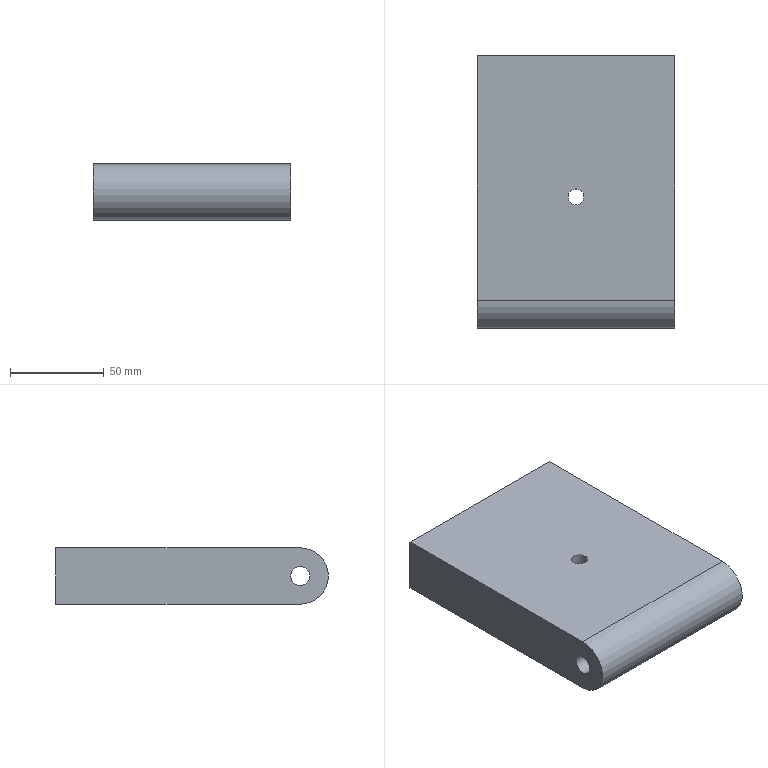Part | STEP file | gslz 2016.10.28-13_id1862_x_t | 1 solid | 8 faces | box 105 x 145.1 x 30 mm | volume 436893 mm3 | plane 5 | cylinder 3 | commonest cylinder face diameters 8.5 x1 10.05 x1 30 x1
STEP:
#1=CARTESIAN_POINT('',(0.,0.,0.));
#2=DIRECTION('',(0.,0.,1.));
#3=DIRECTION('',(1.,0.,0.));
#4=AXIS2_PLACEMENT_3D('',#1,#2,#3);
#5=CARTESIAN_POINT('',(1182.5,600.1,-49.));
#6=VERTEX_POINT('',#5);
#7=CARTESIAN_POINT('',(1182.5,730.2,-49.));
#8=VERTEX_POINT('',#7);
#9=CARTESIAN_POINT('',(1182.5,600.95,-49.));
#10=DIRECTION('',(0.,1.,0.));
#11=VECTOR('',#10,1.);
#12=LINE('',#9,#11);
#13=CARTESIAN_POINT('',(1322.5,601.2,-49.));
#14=DIRECTION('',(0.,0.,-1.));
#15=DIRECTION('',(0.,1.,0.));
#16=AXIS2_PLACEMENT_3D('',#13,#14,#15);
#17=PLANE('',#16);
#18=CARTESIAN_POINT('',(-0.25,-140.));
#19=DIRECTION('',(1.,0.));
#20=VECTOR('',#19,1.);
#21=LINE('',#18,#20);
#22=(GEOMETRIC_REPRESENTATION_CONTEXT(2)PARAMETRIC_REPRESENTATION_CONTEXT()REPRESENTATION_CONTEXT('',''));
#23=DEFINITIONAL_REPRESENTATION('',(#21),#22);
#24=PCURVE('',#17,#23);
#25=CARTESIAN_POINT('',(1182.5,600.95,-69.));
#26=DIRECTION('',(1.,0.,0.));
#27=DIRECTION('',(0.,0.,1.));
#28=AXIS2_PLACEMENT_3D('',#25,#26,#27);
#29=PLANE('',#28);
#30=CARTESIAN_POINT('',(20.,0.));
#31=DIRECTION('',(0.,-1.));
#32=VECTOR('',#31,1.);
#33=LINE('',#30,#32);
#34=(GEOMETRIC_REPRESENTATION_CONTEXT(2)PARAMETRIC_REPRESENTATION_CONTEXT()REPRESENTATION_CONTEXT('',''));
#35=DEFINITIONAL_REPRESENTATION('',(#33),#34);
#36=PCURVE('',#29,#35);
#37=SURFACE_CURVE('',#12,(#24,#36),.PCURVE_S1.);
#38=EDGE_CURVE('',#6,#8,#37,.T.);
#39=ORIENTED_EDGE('',*,*,#38,.F.);
#40=CARTESIAN_POINT('',(1287.5,600.1,-49.));
#41=VERTEX_POINT('',#40);
#42=CARTESIAN_POINT('',(1235.,600.1,-49.));
#43=DIRECTION('',(1.,0.,0.));
#44=VECTOR('',#43,1.);
#45=LINE('',#42,#44);
#46=CARTESIAN_POINT('',(-1.1,-87.5));
#47=DIRECTION('',(0.,1.));
#48=VECTOR('',#47,1.);
#49=LINE('',#46,#48);
#50=(GEOMETRIC_REPRESENTATION_CONTEXT(2)PARAMETRIC_REPRESENTATION_CONTEXT()REPRESENTATION_CONTEXT('',''));
#51=DEFINITIONAL_REPRESENTATION('',(#49),#50);
#52=PCURVE('',#17,#51);
#53=CARTESIAN_POINT('',(1322.5,600.1,-64.));
#54=DIRECTION('',(-1.,0.,0.));
#55=DIRECTION('',(0.,0.,1.));
#56=AXIS2_PLACEMENT_3D('',#53,#54,#55);
#57=CYLINDRICAL_SURFACE('',#56,15.);
#58=CARTESIAN_POINT('',(6.283,87.5));
#59=DIRECTION('',(0.,-1.));
#60=VECTOR('',#59,1.);
#61=LINE('',#58,#60);
#62=(GEOMETRIC_REPRESENTATION_CONTEXT(2)PARAMETRIC_REPRESENTATION_CONTEXT()REPRESENTATION_CONTEXT('',''));
#63=DEFINITIONAL_REPRESENTATION('',(#61),#62);
#64=PCURVE('',#57,#63);
#65=SURFACE_CURVE('',#45,(#52,#64),.PCURVE_S1.);
#66=EDGE_CURVE('',#6,#41,#65,.T.);
#67=ORIENTED_EDGE('',*,*,#66,.T.);
#68=CARTESIAN_POINT('',(1287.5,730.2,-49.));
#69=VERTEX_POINT('',#68);
#70=CARTESIAN_POINT('',(1287.5,600.95,-49.));
#71=DIRECTION('',(0.,-1.,0.));
#72=VECTOR('',#71,1.);
#73=LINE('',#70,#72);
#74=CARTESIAN_POINT('',(-0.25,-35.));
#75=DIRECTION('',(-1.,0.));
#76=VECTOR('',#75,1.);
#77=LINE('',#74,#76);
#78=(GEOMETRIC_REPRESENTATION_CONTEXT(2)PARAMETRIC_REPRESENTATION_CONTEXT()REPRESENTATION_CONTEXT('',''));
#79=DEFINITIONAL_REPRESENTATION('',(#77),#78);
#80=PCURVE('',#17,#79);
#81=CARTESIAN_POINT('',(1287.5,600.95,-69.));
#82=DIRECTION('',(-1.,0.,0.));
#83=DIRECTION('',(0.,0.,1.));
#84=AXIS2_PLACEMENT_3D('',#81,#82,#83);
#85=PLANE('',#84);
#86=CARTESIAN_POINT('',(20.,0.));
#87=DIRECTION('',(0.,-1.));
#88=VECTOR('',#87,1.);
#89=LINE('',#86,#88);
#90=(GEOMETRIC_REPRESENTATION_CONTEXT(2)PARAMETRIC_REPRESENTATION_CONTEXT()REPRESENTATION_CONTEXT('',''));
#91=DEFINITIONAL_REPRESENTATION('',(#89),#90);
#92=PCURVE('',#85,#91);
#93=SURFACE_CURVE('',#73,(#80,#92),.PCURVE_S1.);
#94=EDGE_CURVE('',#69,#41,#93,.T.);
#95=ORIENTED_EDGE('',*,*,#94,.F.);
#96=CARTESIAN_POINT('',(1322.5,730.2,-49.));
#97=DIRECTION('',(-1.,0.,0.));
#98=VECTOR('',#97,1.);
#99=LINE('',#96,#98);
#100=CARTESIAN_POINT('',(129.,0.));
#101=DIRECTION('',(0.,-1.));
#102=VECTOR('',#101,1.);
#103=LINE('',#100,#102);
#104=(GEOMETRIC_REPRESENTATION_CONTEXT(2)PARAMETRIC_REPRESENTATION_CONTEXT()REPRESENTATION_CONTEXT('',''));
#105=DEFINITIONAL_REPRESENTATION('',(#103),#104);
#106=PCURVE('',#17,#105);
#107=CARTESIAN_POINT('',(1322.5,730.2,-34.));
#108=DIRECTION('',(0.,-1.,0.));
#109=DIRECTION('',(-1.,0.,0.));
#110=AXIS2_PLACEMENT_3D('',#107,#108,#109);
#111=PLANE('',#110);
#112=CARTESIAN_POINT('',(0.,15.));
#113=DIRECTION('',(1.,0.));
#114=VECTOR('',#113,1.);
#115=LINE('',#112,#114);
#116=(GEOMETRIC_REPRESENTATION_CONTEXT(2)PARAMETRIC_REPRESENTATION_CONTEXT()REPRESENTATION_CONTEXT('',''));
#117=DEFINITIONAL_REPRESENTATION('',(#115),#116);
#118=PCURVE('',#111,#117);
#119=SURFACE_CURVE('',#99,(#106,#118),.PCURVE_S1.);
#120=EDGE_CURVE('',#69,#8,#119,.T.);
#121=ORIENTED_EDGE('',*,*,#120,.T.);
#122=EDGE_LOOP('',(#39,#67,#95,#121));
#123=FACE_BOUND('',#122,.T.);
#124=CARTESIAN_POINT('',(1230.75,655.1,-49.));
#125=VERTEX_POINT('',#124);
#126=CARTESIAN_POINT('',(1235.,655.1,-49.));
#127=DIRECTION('',(0.,0.,1.));
#128=DIRECTION('',(-1.,0.,0.));
#129=AXIS2_PLACEMENT_3D('',#126,#127,#128);
#130=CIRCLE('',#129,4.25);
#131=CARTESIAN_POINT('',(53.9,-91.75));
#132=CARTESIAN_POINT('',(46.539,-91.75));
#133=CARTESIAN_POINT('',(50.219,-85.375));
#134=CARTESIAN_POINT('',(53.9,-79.));
#135=CARTESIAN_POINT('',(57.581,-85.375));
#136=CARTESIAN_POINT('',(61.261,-91.75));
#137=CARTESIAN_POINT('',(53.9,-91.75));
#138=(BOUNDED_CURVE()B_SPLINE_CURVE(2,(#131,#132,#133,#134,#135,#136,#137),.UNSPECIFIED.,.T.,.F.)B_SPLINE_CURVE_WITH_KNOTS((1,2,2,2,2,1),(-2.094,0.,2.094,4.189,6.283,8.378),.UNSPECIFIED.)CURVE()GEOMETRIC_REPRESENTATION_ITEM()RATIONAL_B_SPLINE_CURVE((1.,0.5,1.,0.5,1.,0.5,1.))REPRESENTATION_ITEM(''));
#139=(GEOMETRIC_REPRESENTATION_CONTEXT(2)PARAMETRIC_REPRESENTATION_CONTEXT()REPRESENTATION_CONTEXT('',''));
#140=DEFINITIONAL_REPRESENTATION('',(#138),#139);
#141=PCURVE('',#17,#140);
#142=CARTESIAN_POINT('',(1235.,655.1,356.));
#143=DIRECTION('',(0.,0.,-1.));
#144=DIRECTION('',(-1.,0.,0.));
#145=AXIS2_PLACEMENT_3D('',#142,#143,#144);
#146=CYLINDRICAL_SURFACE('',#145,4.25);
#147=CARTESIAN_POINT('',(6.283,405.));
#148=DIRECTION('',(-1.,0.));
#149=VECTOR('',#148,1.);
#150=LINE('',#147,#149);
#151=(GEOMETRIC_REPRESENTATION_CONTEXT(2)PARAMETRIC_REPRESENTATION_CONTEXT()REPRESENTATION_CONTEXT('',''));
#152=DEFINITIONAL_REPRESENTATION('',(#150),#151);
#153=PCURVE('',#146,#152);
#154=SURFACE_CURVE('',#130,(#141,#153),.PCURVE_S1.);
#155=EDGE_CURVE('',#125,#125,#154,.T.);
#156=ORIENTED_EDGE('',*,*,#155,.F.);
#157=EDGE_LOOP('',(#156));
#158=FACE_BOUND('',#157,.T.);
#159=ADVANCED_FACE('',(#123,#158),#17,.F.);
#160=CARTESIAN_POINT('',(1287.5,600.1,-79.));
#161=VERTEX_POINT('',#160);
#162=CARTESIAN_POINT('',(1287.5,730.2,-79.));
#163=VERTEX_POINT('',#162);
#164=CARTESIAN_POINT('',(1287.5,600.95,-79.));
#165=DIRECTION('',(0.,1.,0.));
#166=VECTOR('',#165,1.);
#167=LINE('',#164,#166);
#168=CARTESIAN_POINT('',(1322.5,581.2,-79.));
#169=DIRECTION('',(0.,0.,1.));
#170=DIRECTION('',(0.,-1.,0.));
#171=AXIS2_PLACEMENT_3D('',#168,#169,#170);
#172=PLANE('',#171);
#173=CARTESIAN_POINT('',(-19.75,-35.));
#174=DIRECTION('',(-1.,0.));
#175=VECTOR('',#174,1.);
#176=LINE('',#173,#175);
#177=(GEOMETRIC_REPRESENTATION_CONTEXT(2)PARAMETRIC_REPRESENTATION_CONTEXT()REPRESENTATION_CONTEXT('',''));
#178=DEFINITIONAL_REPRESENTATION('',(#176),#177);
#179=PCURVE('',#172,#178);
#180=CARTESIAN_POINT('',(-10.,0.));
#181=DIRECTION('',(0.,1.));
#182=VECTOR('',#181,1.);
#183=LINE('',#180,#182);
#184=(GEOMETRIC_REPRESENTATION_CONTEXT(2)PARAMETRIC_REPRESENTATION_CONTEXT()REPRESENTATION_CONTEXT('',''));
#185=DEFINITIONAL_REPRESENTATION('',(#183),#184);
#186=PCURVE('',#85,#185);
#187=SURFACE_CURVE('',#167,(#179,#186),.PCURVE_S1.);
#188=EDGE_CURVE('',#161,#163,#187,.T.);
#189=ORIENTED_EDGE('',*,*,#188,.F.);
#190=CARTESIAN_POINT('',(1182.5,600.1,-79.));
#191=VERTEX_POINT('',#190);
#192=CARTESIAN_POINT('',(1235.,600.1,-79.));
#193=DIRECTION('',(-1.,0.,0.));
#194=VECTOR('',#193,1.);
#195=LINE('',#192,#194);
#196=CARTESIAN_POINT('',(-18.9,-87.5));
#197=DIRECTION('',(0.,-1.));
#198=VECTOR('',#197,1.);
#199=LINE('',#196,#198);
#200=(GEOMETRIC_REPRESENTATION_CONTEXT(2)PARAMETRIC_REPRESENTATION_CONTEXT()REPRESENTATION_CONTEXT('',''));
#201=DEFINITIONAL_REPRESENTATION('',(#199),#200);
#202=PCURVE('',#172,#201);
#203=CARTESIAN_POINT('',(3.142,87.5));
#204=DIRECTION('',(0.,1.));
#205=VECTOR('',#204,1.);
#206=LINE('',#203,#205);
#207=(GEOMETRIC_REPRESENTATION_CONTEXT(2)PARAMETRIC_REPRESENTATION_CONTEXT()REPRESENTATION_CONTEXT('',''));
#208=DEFINITIONAL_REPRESENTATION('',(#206),#207);
#209=PCURVE('',#57,#208);
#210=SURFACE_CURVE('',#195,(#202,#209),.PCURVE_S1.);
#211=EDGE_CURVE('',#161,#191,#210,.T.);
#212=ORIENTED_EDGE('',*,*,#211,.T.);
#213=CARTESIAN_POINT('',(1182.5,730.2,-79.));
#214=VERTEX_POINT('',#213);
#215=CARTESIAN_POINT('',(1182.5,581.2,-79.));
#216=DIRECTION('',(0.,1.,0.));
#217=VECTOR('',#216,1.);
#218=LINE('',#215,#217);
#219=CARTESIAN_POINT('',(0.,-140.));
#220=DIRECTION('',(-1.,0.));
#221=VECTOR('',#220,1.);
#222=LINE('',#219,#221);
#223=(GEOMETRIC_REPRESENTATION_CONTEXT(2)PARAMETRIC_REPRESENTATION_CONTEXT()REPRESENTATION_CONTEXT('',''));
#224=DEFINITIONAL_REPRESENTATION('',(#222),#223);
#225=PCURVE('',#172,#224);
#226=CARTESIAN_POINT('',(-10.,19.75));
#227=DIRECTION('',(0.,-1.));
#228=VECTOR('',#227,1.);
#229=LINE('',#226,#228);
#230=(GEOMETRIC_REPRESENTATION_CONTEXT(2)PARAMETRIC_REPRESENTATION_CONTEXT()REPRESENTATION_CONTEXT('',''));
#231=DEFINITIONAL_REPRESENTATION('',(#229),#230);
#232=PCURVE('',#29,#231);
#233=SURFACE_CURVE('',#218,(#225,#232),.PCURVE_S1.);
#234=EDGE_CURVE('',#191,#214,#233,.T.);
#235=ORIENTED_EDGE('',*,*,#234,.T.);
#236=CARTESIAN_POINT('',(1322.5,730.2,-79.));
#237=DIRECTION('',(-1.,0.,0.));
#238=VECTOR('',#237,1.);
#239=LINE('',#236,#238);
#240=CARTESIAN_POINT('',(-149.,0.));
#241=DIRECTION('',(0.,-1.));
#242=VECTOR('',#241,1.);
#243=LINE('',#240,#242);
#244=(GEOMETRIC_REPRESENTATION_CONTEXT(2)PARAMETRIC_REPRESENTATION_CONTEXT()REPRESENTATION_CONTEXT('',''));
#245=DEFINITIONAL_REPRESENTATION('',(#243),#244);
#246=PCURVE('',#172,#245);
#247=CARTESIAN_POINT('',(0.,45.));
#248=DIRECTION('',(1.,0.));
#249=VECTOR('',#248,1.);
#250=LINE('',#247,#249);
#251=(GEOMETRIC_REPRESENTATION_CONTEXT(2)PARAMETRIC_REPRESENTATION_CONTEXT()REPRESENTATION_CONTEXT('',''));
#252=DEFINITIONAL_REPRESENTATION('',(#250),#251);
#253=PCURVE('',#111,#252);
#254=SURFACE_CURVE('',#239,(#246,#253),.PCURVE_S1.);
#255=EDGE_CURVE('',#163,#214,#254,.T.);
#256=ORIENTED_EDGE('',*,*,#255,.F.);
#257=EDGE_LOOP('',(#189,#212,#235,#256));
#258=FACE_BOUND('',#257,.T.);
#259=CARTESIAN_POINT('',(1239.25,655.1,-79.));
#260=VERTEX_POINT('',#259);
#261=CARTESIAN_POINT('',(1230.75,655.1,-79.));
#262=VERTEX_POINT('',#261);
#263=CARTESIAN_POINT('',(1235.,655.1,-79.));
#264=DIRECTION('',(0.,0.,-1.));
#265=DIRECTION('',(1.,0.,0.));
#266=AXIS2_PLACEMENT_3D('',#263,#264,#265);
#267=CIRCLE('',#266,4.25);
#268=CARTESIAN_POINT('',(-73.9,-83.25));
#269=CARTESIAN_POINT('',(-66.539,-83.25));
#270=CARTESIAN_POINT('',(-70.219,-89.625));
#271=CARTESIAN_POINT('',(-73.9,-96.));
#272=CARTESIAN_POINT('',(-77.581,-89.625));
#273=CARTESIAN_POINT('',(-81.261,-83.25));
#274=CARTESIAN_POINT('',(-73.9,-83.25));
#275=(BOUNDED_CURVE()B_SPLINE_CURVE(2,(#268,#269,#270,#271,#272,#273,#274),.UNSPECIFIED.,.T.,.F.)B_SPLINE_CURVE_WITH_KNOTS((1,2,2,2,2,1),(-2.094,0.,2.094,4.189,6.283,8.378),.UNSPECIFIED.)CURVE()GEOMETRIC_REPRESENTATION_ITEM()RATIONAL_B_SPLINE_CURVE((1.,0.5,1.,0.5,1.,0.5,1.))REPRESENTATION_ITEM(''));
#276=(GEOMETRIC_REPRESENTATION_CONTEXT(2)PARAMETRIC_REPRESENTATION_CONTEXT()REPRESENTATION_CONTEXT('',''));
#277=DEFINITIONAL_REPRESENTATION('',(#275),#276);
#278=PCURVE('',#172,#277);
#279=CARTESIAN_POINT('',(3.142,435.));
#280=DIRECTION('',(1.,0.));
#281=VECTOR('',#280,1.);
#282=LINE('',#279,#281);
#283=(GEOMETRIC_REPRESENTATION_CONTEXT(2)PARAMETRIC_REPRESENTATION_CONTEXT()REPRESENTATION_CONTEXT('',''));
#284=DEFINITIONAL_REPRESENTATION('',(#282),#283);
#285=PCURVE('',#146,#284);
#286=SURFACE_CURVE('',#267,(#278,#285),.PCURVE_S1.);
#287=EDGE_CURVE('',#260,#262,#286,.T.);
#288=ORIENTED_EDGE('',*,*,#287,.F.);
#289=CARTESIAN_POINT('',(1235.,655.1,-79.));
#290=DIRECTION('',(0.,0.,-1.));
#291=DIRECTION('',(1.,0.,0.));
#292=AXIS2_PLACEMENT_3D('',#289,#290,#291);
#293=CIRCLE('',#292,4.25);
#294=CARTESIAN_POINT('',(-73.9,-83.25));
#295=CARTESIAN_POINT('',(-66.539,-83.25));
#296=CARTESIAN_POINT('',(-70.219,-89.625));
#297=CARTESIAN_POINT('',(-73.9,-96.));
#298=CARTESIAN_POINT('',(-77.581,-89.625));
#299=CARTESIAN_POINT('',(-81.261,-83.25));
#300=CARTESIAN_POINT('',(-73.9,-83.25));
#301=(BOUNDED_CURVE()B_SPLINE_CURVE(2,(#294,#295,#296,#297,#298,#299,#300),.UNSPECIFIED.,.T.,.F.)B_SPLINE_CURVE_WITH_KNOTS((1,2,2,2,2,1),(-2.094,0.,2.094,4.189,6.283,8.378),.UNSPECIFIED.)CURVE()GEOMETRIC_REPRESENTATION_ITEM()RATIONAL_B_SPLINE_CURVE((1.,0.5,1.,0.5,1.,0.5,1.))REPRESENTATION_ITEM(''));
#302=(GEOMETRIC_REPRESENTATION_CONTEXT(2)PARAMETRIC_REPRESENTATION_CONTEXT()REPRESENTATION_CONTEXT('',''));
#303=DEFINITIONAL_REPRESENTATION('',(#301),#302);
#304=PCURVE('',#172,#303);
#305=CARTESIAN_POINT('',(-3.142,435.));
#306=DIRECTION('',(1.,0.));
#307=VECTOR('',#306,1.);
#308=LINE('',#305,#307);
#309=(GEOMETRIC_REPRESENTATION_CONTEXT(2)PARAMETRIC_REPRESENTATION_CONTEXT()REPRESENTATION_CONTEXT('',''));
#310=DEFINITIONAL_REPRESENTATION('',(#308),#309);
#311=PCURVE('',#146,#310);
#312=SURFACE_CURVE('',#293,(#304,#311),.PCURVE_S1.);
#313=EDGE_CURVE('',#262,#260,#312,.T.);
#314=ORIENTED_EDGE('',*,*,#313,.F.);
#315=EDGE_LOOP('',(#288,#314));
#316=FACE_BOUND('',#315,.T.);
#317=ADVANCED_FACE('',(#258,#316),#172,.F.);
#318=CARTESIAN_POINT('',(1287.5,600.1,-64.));
#319=DIRECTION('',(1.,0.,0.));
#320=DIRECTION('',(0.,0.,1.));
#321=AXIS2_PLACEMENT_3D('',#318,#319,#320);
#322=CIRCLE('',#321,15.);
#323=CARTESIAN_POINT('',(20.,-0.85));
#324=CARTESIAN_POINT('',(20.,-26.831));
#325=CARTESIAN_POINT('',(-2.5,-13.84));
#326=CARTESIAN_POINT('',(-25.,-0.85));
#327=CARTESIAN_POINT('',(-2.5,12.14));
#328=CARTESIAN_POINT('',(20.,25.131));
#329=CARTESIAN_POINT('',(20.,-0.85));
#330=(BOUNDED_CURVE()B_SPLINE_CURVE(2,(#323,#324,#325,#326,#327,#328,#329),.UNSPECIFIED.,.T.,.F.)B_SPLINE_CURVE_WITH_KNOTS((1,2,2,2,2,1),(-2.094,0.,2.094,4.189,6.283,8.378),.UNSPECIFIED.)CURVE()GEOMETRIC_REPRESENTATION_ITEM()RATIONAL_B_SPLINE_CURVE((1.,0.5,1.,0.5,1.,0.5,1.))REPRESENTATION_ITEM(''));
#331=(GEOMETRIC_REPRESENTATION_CONTEXT(2)PARAMETRIC_REPRESENTATION_CONTEXT()REPRESENTATION_CONTEXT('',''));
#332=DEFINITIONAL_REPRESENTATION('',(#330),#331);
#333=PCURVE('',#85,#332);
#334=CARTESIAN_POINT('',(6.283,35.));
#335=DIRECTION('',(-1.,0.));
#336=VECTOR('',#335,1.);
#337=LINE('',#334,#336);
#338=(GEOMETRIC_REPRESENTATION_CONTEXT(2)PARAMETRIC_REPRESENTATION_CONTEXT()REPRESENTATION_CONTEXT('',''));
#339=DEFINITIONAL_REPRESENTATION('',(#337),#338);
#340=PCURVE('',#57,#339);
#341=SURFACE_CURVE('',#322,(#333,#340),.PCURVE_S1.);
#342=EDGE_CURVE('',#41,#161,#341,.T.);
#343=ORIENTED_EDGE('',*,*,#342,.T.);
#344=ORIENTED_EDGE('',*,*,#188,.T.);
#345=CARTESIAN_POINT('',(1287.5,730.2,-34.));
#346=DIRECTION('',(0.,0.,-1.));
#347=VECTOR('',#346,1.);
#348=LINE('',#345,#347);
#349=CARTESIAN_POINT('',(35.,129.25));
#350=DIRECTION('',(-1.,0.));
#351=VECTOR('',#350,1.);
#352=LINE('',#349,#351);
#353=(GEOMETRIC_REPRESENTATION_CONTEXT(2)PARAMETRIC_REPRESENTATION_CONTEXT()REPRESENTATION_CONTEXT('',''));
#354=DEFINITIONAL_REPRESENTATION('',(#352),#353);
#355=PCURVE('',#85,#354);
#356=CARTESIAN_POINT('',(35.,0.));
#357=DIRECTION('',(0.,1.));
#358=VECTOR('',#357,1.);
#359=LINE('',#356,#358);
#360=(GEOMETRIC_REPRESENTATION_CONTEXT(2)PARAMETRIC_REPRESENTATION_CONTEXT()REPRESENTATION_CONTEXT('',''));
#361=DEFINITIONAL_REPRESENTATION('',(#359),#360);
#362=PCURVE('',#111,#361);
#363=SURFACE_CURVE('',#348,(#355,#362),.PCURVE_S1.);
#364=EDGE_CURVE('',#69,#163,#363,.T.);
#365=ORIENTED_EDGE('',*,*,#364,.F.);
#366=ORIENTED_EDGE('',*,*,#94,.T.);
#367=EDGE_LOOP('',(#343,#344,#365,#366));
#368=FACE_BOUND('',#367,.T.);
#369=CARTESIAN_POINT('',(1287.5,600.1,-58.975));
#370=VERTEX_POINT('',#369);
#371=CARTESIAN_POINT('',(1287.5,600.1,-64.));
#372=DIRECTION('',(1.,0.,0.));
#373=DIRECTION('',(0.,0.,1.));
#374=AXIS2_PLACEMENT_3D('',#371,#372,#373);
#375=CIRCLE('',#374,5.025);
#376=CARTESIAN_POINT('',(10.025,-0.85));
#377=CARTESIAN_POINT('',(10.025,-9.554));
#378=CARTESIAN_POINT('',(2.488,-5.202));
#379=CARTESIAN_POINT('',(-5.05,-0.85));
#380=CARTESIAN_POINT('',(2.488,3.502));
#381=CARTESIAN_POINT('',(10.025,7.854));
#382=CARTESIAN_POINT('',(10.025,-0.85));
#383=(BOUNDED_CURVE()B_SPLINE_CURVE(2,(#376,#377,#378,#379,#380,#381,#382),.UNSPECIFIED.,.T.,.F.)B_SPLINE_CURVE_WITH_KNOTS((1,2,2,2,2,1),(-2.094,0.,2.094,4.189,6.283,8.378),.UNSPECIFIED.)CURVE()GEOMETRIC_REPRESENTATION_ITEM()RATIONAL_B_SPLINE_CURVE((1.,0.5,1.,0.5,1.,0.5,1.))REPRESENTATION_ITEM(''));
#384=(GEOMETRIC_REPRESENTATION_CONTEXT(2)PARAMETRIC_REPRESENTATION_CONTEXT()REPRESENTATION_CONTEXT('',''));
#385=DEFINITIONAL_REPRESENTATION('',(#383),#384);
#386=PCURVE('',#85,#385);
#387=CARTESIAN_POINT('',(1330.,600.1,-64.));
#388=DIRECTION('',(-1.,0.,0.));
#389=DIRECTION('',(0.,0.,1.));
#390=AXIS2_PLACEMENT_3D('',#387,#388,#389);
#391=CYLINDRICAL_SURFACE('',#390,5.025);
#392=CARTESIAN_POINT('',(6.283,42.5));
#393=DIRECTION('',(-1.,0.));
#394=VECTOR('',#393,1.);
#395=LINE('',#392,#394);
#396=(GEOMETRIC_REPRESENTATION_CONTEXT(2)PARAMETRIC_REPRESENTATION_CONTEXT()REPRESENTATION_CONTEXT('',''));
#397=DEFINITIONAL_REPRESENTATION('',(#395),#396);
#398=PCURVE('',#391,#397);
#399=SURFACE_CURVE('',#375,(#386,#398),.PCURVE_S1.);
#400=EDGE_CURVE('',#370,#370,#399,.T.);
#401=ORIENTED_EDGE('',*,*,#400,.F.);
#402=EDGE_LOOP('',(#401));
#403=FACE_BOUND('',#402,.T.);
#404=ADVANCED_FACE('',(#368,#403),#85,.F.);
#405=ORIENTED_EDGE('',*,*,#234,.F.);
#406=CARTESIAN_POINT('',(1182.5,600.1,-64.));
#407=DIRECTION('',(-1.,0.,0.));
#408=DIRECTION('',(0.,0.,-1.));
#409=AXIS2_PLACEMENT_3D('',#406,#407,#408);
#410=CIRCLE('',#409,15.);
#411=CARTESIAN_POINT('',(-10.,0.85));
#412=CARTESIAN_POINT('',(-10.,26.831));
#413=CARTESIAN_POINT('',(12.5,13.84));
#414=CARTESIAN_POINT('',(35.,0.85));
#415=CARTESIAN_POINT('',(12.5,-12.14));
#416=CARTESIAN_POINT('',(-10.,-25.131));
#417=CARTESIAN_POINT('',(-10.,0.85));
#418=(BOUNDED_CURVE()B_SPLINE_CURVE(2,(#411,#412,#413,#414,#415,#416,#417),.UNSPECIFIED.,.T.,.F.)B_SPLINE_CURVE_WITH_KNOTS((1,2,2,2,2,1),(-2.094,0.,2.094,4.189,6.283,8.378),.UNSPECIFIED.)CURVE()GEOMETRIC_REPRESENTATION_ITEM()RATIONAL_B_SPLINE_CURVE((1.,0.5,1.,0.5,1.,0.5,1.))REPRESENTATION_ITEM(''));
#419=(GEOMETRIC_REPRESENTATION_CONTEXT(2)PARAMETRIC_REPRESENTATION_CONTEXT()REPRESENTATION_CONTEXT('',''));
#420=DEFINITIONAL_REPRESENTATION('',(#418),#419);
#421=PCURVE('',#29,#420);
#422=CARTESIAN_POINT('',(3.142,140.));
#423=DIRECTION('',(1.,0.));
#424=VECTOR('',#423,1.);
#425=LINE('',#422,#424);
#426=(GEOMETRIC_REPRESENTATION_CONTEXT(2)PARAMETRIC_REPRESENTATION_CONTEXT()REPRESENTATION_CONTEXT('',''));
#427=DEFINITIONAL_REPRESENTATION('',(#425),#426);
#428=PCURVE('',#57,#427);
#429=SURFACE_CURVE('',#410,(#421,#428),.PCURVE_S1.);
#430=EDGE_CURVE('',#191,#6,#429,.T.);
#431=ORIENTED_EDGE('',*,*,#430,.T.);
#432=ORIENTED_EDGE('',*,*,#38,.T.);
#433=CARTESIAN_POINT('',(1182.5,730.2,-34.));
#434=DIRECTION('',(0.,0.,1.));
#435=VECTOR('',#434,1.);
#436=LINE('',#433,#435);
#437=CARTESIAN_POINT('',(35.,-129.25));
#438=DIRECTION('',(1.,0.));
#439=VECTOR('',#438,1.);
#440=LINE('',#437,#439);
#441=(GEOMETRIC_REPRESENTATION_CONTEXT(2)PARAMETRIC_REPRESENTATION_CONTEXT()REPRESENTATION_CONTEXT('',''));
#442=DEFINITIONAL_REPRESENTATION('',(#440),#441);
#443=PCURVE('',#29,#442);
#444=CARTESIAN_POINT('',(140.,0.));
#445=DIRECTION('',(0.,-1.));
#446=VECTOR('',#445,1.);
#447=LINE('',#444,#446);
#448=(GEOMETRIC_REPRESENTATION_CONTEXT(2)PARAMETRIC_REPRESENTATION_CONTEXT()REPRESENTATION_CONTEXT('',''));
#449=DEFINITIONAL_REPRESENTATION('',(#447),#448);
#450=PCURVE('',#111,#449);
#451=SURFACE_CURVE('',#436,(#443,#450),.PCURVE_S1.);
#452=EDGE_CURVE('',#214,#8,#451,.T.);
#453=ORIENTED_EDGE('',*,*,#452,.F.);
#454=EDGE_LOOP('',(#405,#431,#432,#453));
#455=FACE_BOUND('',#454,.T.);
#456=CARTESIAN_POINT('',(1182.5,600.1,-69.025));
#457=VERTEX_POINT('',#456);
#458=CARTESIAN_POINT('',(1182.5,600.1,-58.975));
#459=VERTEX_POINT('',#458);
#460=CARTESIAN_POINT('',(1182.5,600.1,-64.));
#461=DIRECTION('',(-1.,0.,0.));
#462=DIRECTION('',(0.,0.,-1.));
#463=AXIS2_PLACEMENT_3D('',#460,#461,#462);
#464=CIRCLE('',#463,5.025);
#465=CARTESIAN_POINT('',(-0.025,0.85));
#466=CARTESIAN_POINT('',(-0.025,9.554));
#467=CARTESIAN_POINT('',(7.513,5.202));
#468=CARTESIAN_POINT('',(15.05,0.85));
#469=CARTESIAN_POINT('',(7.513,-3.502));
#470=CARTESIAN_POINT('',(-0.025,-7.854));
#471=CARTESIAN_POINT('',(-0.025,0.85));
#472=(BOUNDED_CURVE()B_SPLINE_CURVE(2,(#465,#466,#467,#468,#469,#470,#471),.UNSPECIFIED.,.T.,.F.)B_SPLINE_CURVE_WITH_KNOTS((1,2,2,2,2,1),(-2.094,0.,2.094,4.189,6.283,8.378),.UNSPECIFIED.)CURVE()GEOMETRIC_REPRESENTATION_ITEM()RATIONAL_B_SPLINE_CURVE((1.,0.5,1.,0.5,1.,0.5,1.))REPRESENTATION_ITEM(''));
#473=(GEOMETRIC_REPRESENTATION_CONTEXT(2)PARAMETRIC_REPRESENTATION_CONTEXT()REPRESENTATION_CONTEXT('',''));
#474=DEFINITIONAL_REPRESENTATION('',(#472),#473);
#475=PCURVE('',#29,#474);
#476=CARTESIAN_POINT('',(3.142,147.5));
#477=DIRECTION('',(1.,0.));
#478=VECTOR('',#477,1.);
#479=LINE('',#476,#478);
#480=(GEOMETRIC_REPRESENTATION_CONTEXT(2)PARAMETRIC_REPRESENTATION_CONTEXT()REPRESENTATION_CONTEXT('',''));
#481=DEFINITIONAL_REPRESENTATION('',(#479),#480);
#482=PCURVE('',#391,#481);
#483=SURFACE_CURVE('',#464,(#475,#482),.PCURVE_S1.);
#484=EDGE_CURVE('',#457,#459,#483,.T.);
#485=ORIENTED_EDGE('',*,*,#484,.F.);
#486=CARTESIAN_POINT('',(1182.5,600.1,-64.));
#487=DIRECTION('',(-1.,0.,0.));
#488=DIRECTION('',(0.,0.,-1.));
#489=AXIS2_PLACEMENT_3D('',#486,#487,#488);
#490=CIRCLE('',#489,5.025);
#491=CARTESIAN_POINT('',(-0.025,0.85));
#492=CARTESIAN_POINT('',(-0.025,9.554));
#493=CARTESIAN_POINT('',(7.513,5.202));
#494=CARTESIAN_POINT('',(15.05,0.85));
#495=CARTESIAN_POINT('',(7.513,-3.502));
#496=CARTESIAN_POINT('',(-0.025,-7.854));
#497=CARTESIAN_POINT('',(-0.025,0.85));
#498=(BOUNDED_CURVE()B_SPLINE_CURVE(2,(#491,#492,#493,#494,#495,#496,#497),.UNSPECIFIED.,.T.,.F.)B_SPLINE_CURVE_WITH_KNOTS((1,2,2,2,2,1),(-2.094,0.,2.094,4.189,6.283,8.378),.UNSPECIFIED.)CURVE()GEOMETRIC_REPRESENTATION_ITEM()RATIONAL_B_SPLINE_CURVE((1.,0.5,1.,0.5,1.,0.5,1.))REPRESENTATION_ITEM(''));
#499=(GEOMETRIC_REPRESENTATION_CONTEXT(2)PARAMETRIC_REPRESENTATION_CONTEXT()REPRESENTATION_CONTEXT('',''));
#500=DEFINITIONAL_REPRESENTATION('',(#498),#499);
#501=PCURVE('',#29,#500);
#502=CARTESIAN_POINT('',(-3.142,147.5));
#503=DIRECTION('',(1.,0.));
#504=VECTOR('',#503,1.);
#505=LINE('',#502,#504);
#506=(GEOMETRIC_REPRESENTATION_CONTEXT(2)PARAMETRIC_REPRESENTATION_CONTEXT()REPRESENTATION_CONTEXT('',''));
#507=DEFINITIONAL_REPRESENTATION('',(#505),#506);
#508=PCURVE('',#391,#507);
#509=SURFACE_CURVE('',#490,(#501,#508),.PCURVE_S1.);
#510=EDGE_CURVE('',#459,#457,#509,.T.);
#511=ORIENTED_EDGE('',*,*,#510,.F.);
#512=EDGE_LOOP('',(#485,#511));
#513=FACE_BOUND('',#512,.T.);
#514=ADVANCED_FACE('',(#455,#513),#29,.F.);
#515=ORIENTED_EDGE('',*,*,#255,.T.);
#516=ORIENTED_EDGE('',*,*,#452,.T.);
#517=ORIENTED_EDGE('',*,*,#120,.F.);
#518=ORIENTED_EDGE('',*,*,#364,.T.);
#519=EDGE_LOOP('',(#515,#516,#517,#518));
#520=FACE_BOUND('',#519,.T.);
#521=ADVANCED_FACE('',(#520),#111,.F.);
#522=ORIENTED_EDGE('',*,*,#430,.F.);
#523=ORIENTED_EDGE('',*,*,#211,.F.);
#524=ORIENTED_EDGE('',*,*,#342,.F.);
#525=ORIENTED_EDGE('',*,*,#66,.F.);
#526=EDGE_LOOP('',(#522,#523,#524,#525));
#527=FACE_BOUND('',#526,.T.);
#528=ADVANCED_FACE('',(#527),#57,.T.);
#529=ORIENTED_EDGE('',*,*,#510,.F.);
#530=CARTESIAN_POINT('',(1287.5,600.1,-58.975));
#531=CARTESIAN_POINT('',(1182.5,600.1,-58.975));
#532=B_SPLINE_CURVE_WITH_KNOTS('',1,(#530,#531),.UNSPECIFIED.,.F.,.F.,(2,2),(42.5,147.5),.PIECEWISE_BEZIER_KNOTS.);
#533=CARTESIAN_POINT('',(0.,0.));
#534=DIRECTION('',(0.,1.));
#535=VECTOR('',#534,1.);
#536=LINE('',#533,#535);
#537=(GEOMETRIC_REPRESENTATION_CONTEXT(2)PARAMETRIC_REPRESENTATION_CONTEXT()REPRESENTATION_CONTEXT('',''));
#538=DEFINITIONAL_REPRESENTATION('',(#536),#537);
#539=PCURVE('',#391,#538);
#540=CARTESIAN_POINT('',(6.283,0.));
#541=DIRECTION('',(0.,1.));
#542=VECTOR('',#541,1.);
#543=LINE('',#540,#542);
#544=(GEOMETRIC_REPRESENTATION_CONTEXT(2)PARAMETRIC_REPRESENTATION_CONTEXT()REPRESENTATION_CONTEXT('',''));
#545=DEFINITIONAL_REPRESENTATION('',(#543),#544);
#546=PCURVE('',#391,#545);
#547=SEAM_CURVE('',#532,(#539,#546),.PCURVE_S1.);
#548=EDGE_CURVE('',#370,#459,#547,.T.);
#549=ORIENTED_EDGE('',*,*,#548,.F.);
#550=ORIENTED_EDGE('',*,*,#400,.F.);
#551=ORIENTED_EDGE('',*,*,#548,.T.);
#552=ORIENTED_EDGE('',*,*,#484,.F.);
#553=EDGE_LOOP('',(#529,#549,#550,#551,#552));
#554=FACE_BOUND('',#553,.F.);
#555=ADVANCED_FACE('',(#554),#391,.F.);
#556=ORIENTED_EDGE('',*,*,#313,.F.);
#557=CARTESIAN_POINT('',(1230.75,655.1,-49.));
#558=CARTESIAN_POINT('',(1230.75,655.1,-79.));
#559=B_SPLINE_CURVE_WITH_KNOTS('',1,(#557,#558),.UNSPECIFIED.,.F.,.F.,(2,2),(405.,435.),.PIECEWISE_BEZIER_KNOTS.);
#560=CARTESIAN_POINT('',(0.,0.));
#561=DIRECTION('',(0.,1.));
#562=VECTOR('',#561,1.);
#563=LINE('',#560,#562);
#564=(GEOMETRIC_REPRESENTATION_CONTEXT(2)PARAMETRIC_REPRESENTATION_CONTEXT()REPRESENTATION_CONTEXT('',''));
#565=DEFINITIONAL_REPRESENTATION('',(#563),#564);
#566=PCURVE('',#146,#565);
#567=CARTESIAN_POINT('',(6.283,0.));
#568=DIRECTION('',(0.,1.));
#569=VECTOR('',#568,1.);
#570=LINE('',#567,#569);
#571=(GEOMETRIC_REPRESENTATION_CONTEXT(2)PARAMETRIC_REPRESENTATION_CONTEXT()REPRESENTATION_CONTEXT('',''));
#572=DEFINITIONAL_REPRESENTATION('',(#570),#571);
#573=PCURVE('',#146,#572);
#574=SEAM_CURVE('',#559,(#566,#573),.PCURVE_S1.);
#575=EDGE_CURVE('',#125,#262,#574,.T.);
#576=ORIENTED_EDGE('',*,*,#575,.F.);
#577=ORIENTED_EDGE('',*,*,#155,.F.);
#578=ORIENTED_EDGE('',*,*,#575,.T.);
#579=ORIENTED_EDGE('',*,*,#287,.F.);
#580=EDGE_LOOP('',(#556,#576,#577,#578,#579));
#581=FACE_BOUND('',#580,.F.);
#582=ADVANCED_FACE('',(#581),#146,.F.);
#583=CLOSED_SHELL('',(#159,#317,#404,#514,#521,#528,#555,#582));
#584=MANIFOLD_SOLID_BREP('',#583);
#585=(LENGTH_UNIT()NAMED_UNIT(*)SI_UNIT(.MILLI.,.METRE.));
#586=UNCERTAINTY_MEASURE_WITH_UNIT(LENGTH_MEASURE(0.000002),#585,'','');
#587=(NAMED_UNIT(*)PLANE_ANGLE_UNIT()SI_UNIT($,.RADIAN.));
#588=(NAMED_UNIT(*)SI_UNIT($,.STERADIAN.)SOLID_ANGLE_UNIT());
#589=(GEOMETRIC_REPRESENTATION_CONTEXT(3)GLOBAL_UNCERTAINTY_ASSIGNED_CONTEXT((#586))GLOBAL_UNIT_ASSIGNED_CONTEXT((#585,#587,#588))REPRESENTATION_CONTEXT('',''));
#590=ADVANCED_BREP_SHAPE_REPRESENTATION('',(#4,#584),#589);